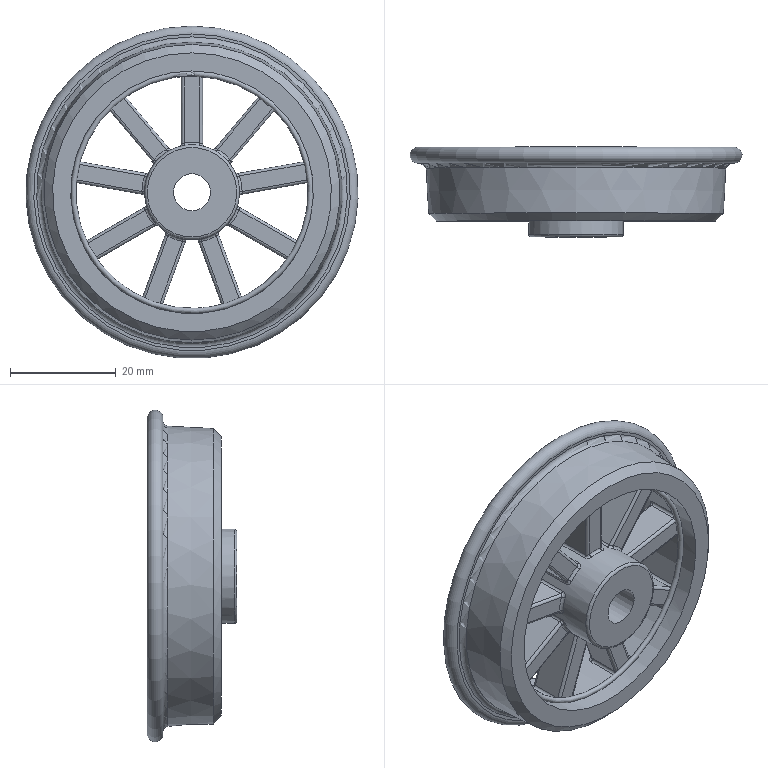Part | STEP file | 2-04.1 | 1 solid | 232 faces | box 63 x 17 x 63 mm | volume 20551 mm3 | cylinder 75 | spline 72 | torus 42 | plane 41 | cone 2 | commonest cylinder face diameters 1 x72 7 x1 18 x1 46 x1